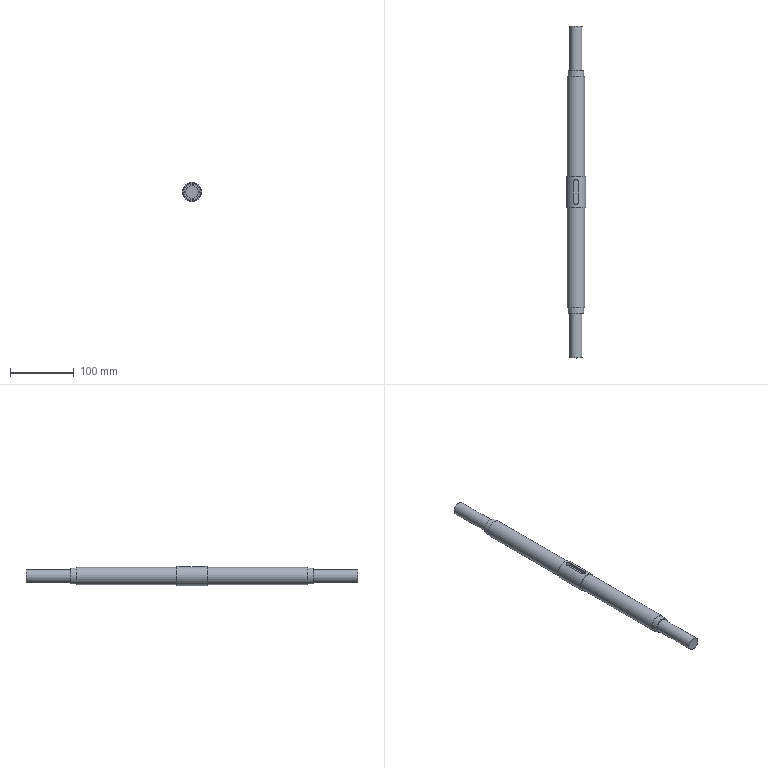Part | NX | features DATUM_CSYS 3, SKETCH 2, EXTRUDE 1, SWP104 1 | 1 solid | 20 faces | box 30 x 520 x 30 mm | volume 265320 mm3 | plane 11 | cylinder 9 | commonest cylinder face diameters 8 x2 20 x2 25 x2 27 x2 30 x1
STEP:
#1=CARTESIAN_POINT('',(0.,235.,15.));
#2=VERTEX_POINT('',#1);
#3=CARTESIAN_POINT('',(0.,235.,0.));
#4=DIRECTION('',(0.,1.,0.));
#5=DIRECTION('',(0.,0.,1.));
#6=AXIS2_PLACEMENT_3D('',#3,#4,#5);
#7=CIRCLE('',#6,15.);
#8=EDGE_CURVE('',#2,#2,#7,.T.);
#9=ORIENTED_EDGE('',*,*,#8,.T.);
#10=EDGE_LOOP('',(#9));
#11=FACE_BOUND('',#10,.T.);
#12=CARTESIAN_POINT('',(0.,285.,15.));
#13=VERTEX_POINT('',#12);
#14=CARTESIAN_POINT('',(0.,285.,0.));
#15=DIRECTION('',(0.,1.,0.));
#16=DIRECTION('',(0.,0.,1.));
#17=AXIS2_PLACEMENT_3D('',#14,#15,#16);
#18=CIRCLE('',#17,15.);
#19=EDGE_CURVE('',#13,#13,#18,.T.);
#20=ORIENTED_EDGE('',*,*,#19,.F.);
#21=EDGE_LOOP('',(#20));
#22=FACE_BOUND('',#21,.T.);
#23=CARTESIAN_POINT('',(-4.,276.,14.457));
#24=VERTEX_POINT('',#23);
#25=CARTESIAN_POINT('',(-4.,244.,14.457));
#26=VERTEX_POINT('',#25);
#27=CARTESIAN_POINT('',(-4.,0.,14.457));
#28=DIRECTION('',(0.,1.,0.));
#29=VECTOR('',#28,1000.);
#30=LINE('',#27,#29);
#31=EDGE_CURVE('',#24,#26,#30,.F.);
#32=ORIENTED_EDGE('',*,*,#31,.F.);
#33=CARTESIAN_POINT('',(4.,276.,14.457));
#34=VERTEX_POINT('',#33);
#35=CARTESIAN_POINT('',(4.,276.,14.457));
#36=CARTESIAN_POINT('',(4.,277.062,14.457));
#37=CARTESIAN_POINT('',(3.133,279.126,14.733));
#38=CARTESIAN_POINT('',(0.005849,280.437,15.133));
#39=CARTESIAN_POINT('',(-3.134,279.128,14.734));
#40=CARTESIAN_POINT('',(-4.,277.062,14.457));
#41=CARTESIAN_POINT('',(-4.,276.,14.457));
#42=B_SPLINE_CURVE_WITH_KNOTS('',3,(#35,#36,#37,#38,#39,#40,#41),.UNSPECIFIED.,.F.,.F.,(4,1,1,1,4),(0.,0.00314,0.006279,0.009419,0.01256),.UNSPECIFIED.);
#43=EDGE_CURVE('',#34,#24,#42,.T.);
#44=ORIENTED_EDGE('',*,*,#43,.F.);
#45=CARTESIAN_POINT('',(4.,244.,14.457));
#46=VERTEX_POINT('',#45);
#47=CARTESIAN_POINT('',(4.,0.,14.457));
#48=DIRECTION('',(0.,1.,0.));
#49=VECTOR('',#48,1000.);
#50=LINE('',#47,#49);
#51=EDGE_CURVE('',#46,#34,#50,.T.);
#52=ORIENTED_EDGE('',*,*,#51,.F.);
#53=CARTESIAN_POINT('',(-4.,244.,14.457));
#54=CARTESIAN_POINT('',(-4.,242.938,14.457));
#55=CARTESIAN_POINT('',(-3.133,240.874,14.733));
#56=CARTESIAN_POINT('',(-0.005849,239.563,15.133));
#57=CARTESIAN_POINT('',(3.134,240.872,14.734));
#58=CARTESIAN_POINT('',(4.,242.938,14.457));
#59=CARTESIAN_POINT('',(4.,244.,14.457));
#60=B_SPLINE_CURVE_WITH_KNOTS('',3,(#53,#54,#55,#56,#57,#58,#59),.UNSPECIFIED.,.F.,.F.,(4,1,1,1,4),(0.,0.00314,0.006279,0.009419,0.01256),.UNSPECIFIED.);
#61=EDGE_CURVE('',#26,#46,#60,.T.);
#62=ORIENTED_EDGE('',*,*,#61,.F.);
#63=EDGE_LOOP('',(#32,#44,#52,#62));
#64=FACE_BOUND('',#63,.T.);
#65=CARTESIAN_POINT('',(0.,0.,0.));
#66=DIRECTION('',(0.,1.,0.));
#67=DIRECTION('',(0.,0.,1.));
#68=AXIS2_PLACEMENT_3D('',#65,#66,#67);
#69=CYLINDRICAL_SURFACE('',#68,15.);
#70=ADVANCED_FACE('',(#11,#22,#64),#69,.T.);
#71=CARTESIAN_POINT('',(0.,0.,10.));
#72=VERTEX_POINT('',#71);
#73=CARTESIAN_POINT('',(0.,0.,0.));
#74=DIRECTION('',(0.,1.,0.));
#75=DIRECTION('',(0.,0.,1.));
#76=AXIS2_PLACEMENT_3D('',#73,#74,#75);
#77=CIRCLE('',#76,10.);
#78=EDGE_CURVE('',#72,#72,#77,.T.);
#79=ORIENTED_EDGE('',*,*,#78,.F.);
#80=EDGE_LOOP('',(#79));
#81=FACE_BOUND('',#80,.T.);
#82=CARTESIAN_POINT('',(0.,0.,0.));
#83=DIRECTION('',(0.,1.,0.));
#84=DIRECTION('',(0.,0.,1.));
#85=AXIS2_PLACEMENT_3D('',#82,#83,#84);
#86=PLANE('',#85);
#87=ADVANCED_FACE('',(#81),#86,.F.);
#88=CARTESIAN_POINT('',(0.,520.,10.));
#89=VERTEX_POINT('',#88);
#90=CARTESIAN_POINT('',(0.,520.,0.));
#91=DIRECTION('',(0.,1.,0.));
#92=DIRECTION('',(0.,0.,1.));
#93=AXIS2_PLACEMENT_3D('',#90,#91,#92);
#94=CIRCLE('',#93,10.);
#95=EDGE_CURVE('',#89,#89,#94,.T.);
#96=ORIENTED_EDGE('',*,*,#95,.T.);
#97=EDGE_LOOP('',(#96));
#98=FACE_BOUND('',#97,.T.);
#99=CARTESIAN_POINT('',(0.,520.,0.));
#100=DIRECTION('',(0.,1.,0.));
#101=DIRECTION('',(0.,0.,1.));
#102=AXIS2_PLACEMENT_3D('',#99,#100,#101);
#103=PLANE('',#102);
#104=ADVANCED_FACE('',(#98),#103,.T.);
#105=ORIENTED_EDGE('',*,*,#95,.F.);
#106=EDGE_LOOP('',(#105));
#107=FACE_BOUND('',#106,.T.);
#108=CARTESIAN_POINT('',(0.,450.,10.));
#109=VERTEX_POINT('',#108);
#110=CARTESIAN_POINT('',(0.,450.,0.));
#111=DIRECTION('',(0.,1.,0.));
#112=DIRECTION('',(0.,0.,1.));
#113=AXIS2_PLACEMENT_3D('',#110,#111,#112);
#114=CIRCLE('',#113,10.);
#115=EDGE_CURVE('',#109,#109,#114,.T.);
#116=ORIENTED_EDGE('',*,*,#115,.T.);
#117=EDGE_LOOP('',(#116));
#118=FACE_BOUND('',#117,.T.);
#119=CARTESIAN_POINT('',(0.,0.,0.));
#120=DIRECTION('',(0.,1.,0.));
#121=DIRECTION('',(0.,0.,1.));
#122=AXIS2_PLACEMENT_3D('',#119,#120,#121);
#123=CYLINDRICAL_SURFACE('',#122,10.);
#124=ADVANCED_FACE('',(#107,#118),#123,.T.);
#125=ORIENTED_EDGE('',*,*,#115,.F.);
#126=EDGE_LOOP('',(#125));
#127=FACE_BOUND('',#126,.T.);
#128=CARTESIAN_POINT('',(0.,450.,12.5));
#129=VERTEX_POINT('',#128);
#130=CARTESIAN_POINT('',(0.,450.,0.));
#131=DIRECTION('',(0.,1.,0.));
#132=DIRECTION('',(0.,0.,1.));
#133=AXIS2_PLACEMENT_3D('',#130,#131,#132);
#134=CIRCLE('',#133,12.5);
#135=EDGE_CURVE('',#129,#129,#134,.T.);
#136=ORIENTED_EDGE('',*,*,#135,.T.);
#137=EDGE_LOOP('',(#136));
#138=FACE_BOUND('',#137,.T.);
#139=CARTESIAN_POINT('',(-12.5,450.,0.));
#140=DIRECTION('',(0.,-1.,0.));
#141=DIRECTION('',(0.,0.,-1.));
#142=AXIS2_PLACEMENT_3D('',#139,#140,#141);
#143=PLANE('',#142);
#144=ADVANCED_FACE('',(#127,#138),#143,.F.);
#145=ORIENTED_EDGE('',*,*,#135,.F.);
#146=EDGE_LOOP('',(#145));
#147=FACE_BOUND('',#146,.T.);
#148=CARTESIAN_POINT('',(0.,441.,12.5));
#149=VERTEX_POINT('',#148);
#150=CARTESIAN_POINT('',(0.,441.,0.));
#151=DIRECTION('',(0.,1.,0.));
#152=DIRECTION('',(0.,0.,1.));
#153=AXIS2_PLACEMENT_3D('',#150,#151,#152);
#154=CIRCLE('',#153,12.5);
#155=EDGE_CURVE('',#149,#149,#154,.T.);
#156=ORIENTED_EDGE('',*,*,#155,.T.);
#157=EDGE_LOOP('',(#156));
#158=FACE_BOUND('',#157,.T.);
#159=CARTESIAN_POINT('',(0.,0.,0.));
#160=DIRECTION('',(0.,1.,0.));
#161=DIRECTION('',(0.,0.,1.));
#162=AXIS2_PLACEMENT_3D('',#159,#160,#161);
#163=CYLINDRICAL_SURFACE('',#162,12.5);
#164=ADVANCED_FACE('',(#147,#158),#163,.T.);
#165=ORIENTED_EDGE('',*,*,#155,.F.);
#166=EDGE_LOOP('',(#165));
#167=FACE_BOUND('',#166,.T.);
#168=CARTESIAN_POINT('',(0.,441.,13.5));
#169=VERTEX_POINT('',#168);
#170=CARTESIAN_POINT('',(0.,441.,0.));
#171=DIRECTION('',(0.,1.,0.));
#172=DIRECTION('',(0.,0.,1.));
#173=AXIS2_PLACEMENT_3D('',#170,#171,#172);
#174=CIRCLE('',#173,13.5);
#175=EDGE_CURVE('',#169,#169,#174,.T.);
#176=ORIENTED_EDGE('',*,*,#175,.T.);
#177=EDGE_LOOP('',(#176));
#178=FACE_BOUND('',#177,.T.);
#179=CARTESIAN_POINT('',(-13.5,441.,0.));
#180=DIRECTION('',(0.,-1.,0.));
#181=DIRECTION('',(0.,0.,-1.));
#182=AXIS2_PLACEMENT_3D('',#179,#180,#181);
#183=PLANE('',#182);
#184=ADVANCED_FACE('',(#167,#178),#183,.F.);
#185=ORIENTED_EDGE('',*,*,#175,.F.);
#186=EDGE_LOOP('',(#185));
#187=FACE_BOUND('',#186,.T.);
#188=CARTESIAN_POINT('',(0.,285.,13.5));
#189=VERTEX_POINT('',#188);
#190=CARTESIAN_POINT('',(0.,285.,0.));
#191=DIRECTION('',(0.,1.,0.));
#192=DIRECTION('',(0.,0.,1.));
#193=AXIS2_PLACEMENT_3D('',#190,#191,#192);
#194=CIRCLE('',#193,13.5);
#195=EDGE_CURVE('',#189,#189,#194,.T.);
#196=ORIENTED_EDGE('',*,*,#195,.T.);
#197=EDGE_LOOP('',(#196));
#198=FACE_BOUND('',#197,.T.);
#199=CARTESIAN_POINT('',(0.,0.,0.));
#200=DIRECTION('',(0.,1.,0.));
#201=DIRECTION('',(0.,0.,1.));
#202=AXIS2_PLACEMENT_3D('',#199,#200,#201);
#203=CYLINDRICAL_SURFACE('',#202,13.5);
#204=ADVANCED_FACE('',(#187,#198),#203,.T.);
#205=ORIENTED_EDGE('',*,*,#195,.F.);
#206=EDGE_LOOP('',(#205));
#207=FACE_BOUND('',#206,.T.);
#208=ORIENTED_EDGE('',*,*,#19,.T.);
#209=EDGE_LOOP('',(#208));
#210=FACE_BOUND('',#209,.T.);
#211=CARTESIAN_POINT('',(-15.,285.,0.));
#212=DIRECTION('',(0.,-1.,0.));
#213=DIRECTION('',(0.,0.,-1.));
#214=AXIS2_PLACEMENT_3D('',#211,#212,#213);
#215=PLANE('',#214);
#216=ADVANCED_FACE('',(#207,#210),#215,.F.);
#217=ORIENTED_EDGE('',*,*,#8,.F.);
#218=EDGE_LOOP('',(#217));
#219=FACE_BOUND('',#218,.T.);
#220=CARTESIAN_POINT('',(0.,235.,13.5));
#221=VERTEX_POINT('',#220);
#222=CARTESIAN_POINT('',(0.,235.,0.));
#223=DIRECTION('',(0.,1.,0.));
#224=DIRECTION('',(0.,0.,1.));
#225=AXIS2_PLACEMENT_3D('',#222,#223,#224);
#226=CIRCLE('',#225,13.5);
#227=EDGE_CURVE('',#221,#221,#226,.T.);
#228=ORIENTED_EDGE('',*,*,#227,.T.);
#229=EDGE_LOOP('',(#228));
#230=FACE_BOUND('',#229,.T.);
#231=CARTESIAN_POINT('',(-13.5,235.,0.));
#232=DIRECTION('',(0.,1.,0.));
#233=DIRECTION('',(0.,0.,1.));
#234=AXIS2_PLACEMENT_3D('',#231,#232,#233);
#235=PLANE('',#234);
#236=ADVANCED_FACE('',(#219,#230),#235,.F.);
#237=ORIENTED_EDGE('',*,*,#227,.F.);
#238=EDGE_LOOP('',(#237));
#239=FACE_BOUND('',#238,.T.);
#240=CARTESIAN_POINT('',(0.,79.,13.5));
#241=VERTEX_POINT('',#240);
#242=CARTESIAN_POINT('',(0.,79.,0.));
#243=DIRECTION('',(0.,1.,0.));
#244=DIRECTION('',(0.,0.,1.));
#245=AXIS2_PLACEMENT_3D('',#242,#243,#244);
#246=CIRCLE('',#245,13.5);
#247=EDGE_CURVE('',#241,#241,#246,.T.);
#248=ORIENTED_EDGE('',*,*,#247,.T.);
#249=EDGE_LOOP('',(#248));
#250=FACE_BOUND('',#249,.T.);
#251=CARTESIAN_POINT('',(0.,0.,0.));
#252=DIRECTION('',(0.,1.,0.));
#253=DIRECTION('',(0.,0.,1.));
#254=AXIS2_PLACEMENT_3D('',#251,#252,#253);
#255=CYLINDRICAL_SURFACE('',#254,13.5);
#256=ADVANCED_FACE('',(#239,#250),#255,.T.);
#257=ORIENTED_EDGE('',*,*,#247,.F.);
#258=EDGE_LOOP('',(#257));
#259=FACE_BOUND('',#258,.T.);
#260=CARTESIAN_POINT('',(0.,79.,12.5));
#261=VERTEX_POINT('',#260);
#262=CARTESIAN_POINT('',(0.,79.,0.));
#263=DIRECTION('',(0.,1.,0.));
#264=DIRECTION('',(0.,0.,1.));
#265=AXIS2_PLACEMENT_3D('',#262,#263,#264);
#266=CIRCLE('',#265,12.5);
#267=EDGE_CURVE('',#261,#261,#266,.T.);
#268=ORIENTED_EDGE('',*,*,#267,.T.);
#269=EDGE_LOOP('',(#268));
#270=FACE_BOUND('',#269,.T.);
#271=CARTESIAN_POINT('',(-12.5,79.,0.));
#272=DIRECTION('',(0.,1.,0.));
#273=DIRECTION('',(0.,0.,1.));
#274=AXIS2_PLACEMENT_3D('',#271,#272,#273);
#275=PLANE('',#274);
#276=ADVANCED_FACE('',(#259,#270),#275,.F.);
#277=ORIENTED_EDGE('',*,*,#267,.F.);
#278=EDGE_LOOP('',(#277));
#279=FACE_BOUND('',#278,.T.);
#280=CARTESIAN_POINT('',(0.,70.,12.5));
#281=VERTEX_POINT('',#280);
#282=CARTESIAN_POINT('',(0.,70.,0.));
#283=DIRECTION('',(0.,1.,0.));
#284=DIRECTION('',(0.,0.,1.));
#285=AXIS2_PLACEMENT_3D('',#282,#283,#284);
#286=CIRCLE('',#285,12.5);
#287=EDGE_CURVE('',#281,#281,#286,.T.);
#288=ORIENTED_EDGE('',*,*,#287,.T.);
#289=EDGE_LOOP('',(#288));
#290=FACE_BOUND('',#289,.T.);
#291=CARTESIAN_POINT('',(0.,0.,0.));
#292=DIRECTION('',(0.,1.,0.));
#293=DIRECTION('',(0.,0.,1.));
#294=AXIS2_PLACEMENT_3D('',#291,#292,#293);
#295=CYLINDRICAL_SURFACE('',#294,12.5);
#296=ADVANCED_FACE('',(#279,#290),#295,.T.);
#297=ORIENTED_EDGE('',*,*,#287,.F.);
#298=EDGE_LOOP('',(#297));
#299=FACE_BOUND('',#298,.T.);
#300=CARTESIAN_POINT('',(0.,70.,10.));
#301=VERTEX_POINT('',#300);
#302=CARTESIAN_POINT('',(0.,70.,0.));
#303=DIRECTION('',(0.,1.,0.));
#304=DIRECTION('',(0.,0.,1.));
#305=AXIS2_PLACEMENT_3D('',#302,#303,#304);
#306=CIRCLE('',#305,10.);
#307=EDGE_CURVE('',#301,#301,#306,.T.);
#308=ORIENTED_EDGE('',*,*,#307,.T.);
#309=EDGE_LOOP('',(#308));
#310=FACE_BOUND('',#309,.T.);
#311=CARTESIAN_POINT('',(-10.,70.,0.));
#312=DIRECTION('',(0.,1.,0.));
#313=DIRECTION('',(0.,0.,1.));
#314=AXIS2_PLACEMENT_3D('',#311,#312,#313);
#315=PLANE('',#314);
#316=ADVANCED_FACE('',(#299,#310),#315,.F.);
#317=ORIENTED_EDGE('',*,*,#307,.F.);
#318=EDGE_LOOP('',(#317));
#319=FACE_BOUND('',#318,.T.);
#320=ORIENTED_EDGE('',*,*,#78,.T.);
#321=EDGE_LOOP('',(#320));
#322=FACE_BOUND('',#321,.T.);
#323=CARTESIAN_POINT('',(0.,0.,0.));
#324=DIRECTION('',(0.,1.,0.));
#325=DIRECTION('',(0.,0.,1.));
#326=AXIS2_PLACEMENT_3D('',#323,#324,#325);
#327=CYLINDRICAL_SURFACE('',#326,10.);
#328=ADVANCED_FACE('',(#319,#322),#327,.T.);
#329=ORIENTED_EDGE('',*,*,#31,.T.);
#330=CARTESIAN_POINT('',(-4.,244.,10.));
#331=VERTEX_POINT('',#330);
#332=CARTESIAN_POINT('',(-4.,244.,32.));
#333=DIRECTION('',(0.,0.,-1.));
#334=VECTOR('',#333,1000.);
#335=LINE('',#332,#334);
#336=EDGE_CURVE('',#331,#26,#335,.F.);
#337=ORIENTED_EDGE('',*,*,#336,.F.);
#338=CARTESIAN_POINT('',(-4.,276.,10.));
#339=VERTEX_POINT('',#338);
#340=CARTESIAN_POINT('',(-4.,276.,10.));
#341=DIRECTION('',(0.,-1.,0.));
#342=VECTOR('',#341,1000.);
#343=LINE('',#340,#342);
#344=EDGE_CURVE('',#331,#339,#343,.F.);
#345=ORIENTED_EDGE('',*,*,#344,.T.);
#346=CARTESIAN_POINT('',(-4.,276.,32.));
#347=DIRECTION('',(0.,0.,-1.));
#348=VECTOR('',#347,1000.);
#349=LINE('',#346,#348);
#350=EDGE_CURVE('',#339,#24,#349,.F.);
#351=ORIENTED_EDGE('',*,*,#350,.T.);
#352=EDGE_LOOP('',(#329,#337,#345,#351));
#353=FACE_BOUND('',#352,.T.);
#354=CARTESIAN_POINT('',(-4.,276.,32.));
#355=DIRECTION('',(1.,0.,0.));
#356=DIRECTION('',(0.,1.,0.));
#357=AXIS2_PLACEMENT_3D('',#354,#355,#356);
#358=PLANE('',#357);
#359=ADVANCED_FACE('',(#353),#358,.T.);
#360=ORIENTED_EDGE('',*,*,#61,.T.);
#361=CARTESIAN_POINT('',(4.,244.,10.));
#362=VERTEX_POINT('',#361);
#363=CARTESIAN_POINT('',(4.,244.,32.));
#364=DIRECTION('',(0.,0.,-1.));
#365=VECTOR('',#364,1000.);
#366=LINE('',#363,#365);
#367=EDGE_CURVE('',#362,#46,#366,.F.);
#368=ORIENTED_EDGE('',*,*,#367,.F.);
#369=CARTESIAN_POINT('',(0.,244.,10.));
#370=DIRECTION('',(0.,0.,1.));
#371=DIRECTION('',(1.,0.,0.));
#372=AXIS2_PLACEMENT_3D('',#369,#370,#371);
#373=CIRCLE('',#372,4.);
#374=EDGE_CURVE('',#362,#331,#373,.F.);
#375=ORIENTED_EDGE('',*,*,#374,.T.);
#376=ORIENTED_EDGE('',*,*,#336,.T.);
#377=EDGE_LOOP('',(#360,#368,#375,#376));
#378=FACE_BOUND('',#377,.T.);
#379=CARTESIAN_POINT('',(0.,244.,32.));
#380=DIRECTION('',(0.,0.,-1.));
#381=DIRECTION('',(-1.,0.,0.));
#382=AXIS2_PLACEMENT_3D('',#379,#380,#381);
#383=CYLINDRICAL_SURFACE('',#382,4.);
#384=ADVANCED_FACE('',(#378),#383,.F.);
#385=ORIENTED_EDGE('',*,*,#51,.T.);
#386=CARTESIAN_POINT('',(4.,276.,10.));
#387=VERTEX_POINT('',#386);
#388=CARTESIAN_POINT('',(4.,276.,32.));
#389=DIRECTION('',(0.,0.,-1.));
#390=VECTOR('',#389,1000.);
#391=LINE('',#388,#390);
#392=EDGE_CURVE('',#387,#34,#391,.F.);
#393=ORIENTED_EDGE('',*,*,#392,.F.);
#394=CARTESIAN_POINT('',(4.,244.,10.));
#395=DIRECTION('',(0.,1.,0.));
#396=VECTOR('',#395,1000.);
#397=LINE('',#394,#396);
#398=EDGE_CURVE('',#387,#362,#397,.F.);
#399=ORIENTED_EDGE('',*,*,#398,.T.);
#400=ORIENTED_EDGE('',*,*,#367,.T.);
#401=EDGE_LOOP('',(#385,#393,#399,#400));
#402=FACE_BOUND('',#401,.T.);
#403=CARTESIAN_POINT('',(4.,244.,32.));
#404=DIRECTION('',(-1.,0.,0.));
#405=DIRECTION('',(0.,0.,1.));
#406=AXIS2_PLACEMENT_3D('',#403,#404,#405);
#407=PLANE('',#406);
#408=ADVANCED_FACE('',(#402),#407,.T.);
#409=ORIENTED_EDGE('',*,*,#43,.T.);
#410=ORIENTED_EDGE('',*,*,#350,.F.);
#411=CARTESIAN_POINT('',(0.,276.,10.));
#412=DIRECTION('',(0.,0.,1.));
#413=DIRECTION('',(1.,0.,0.));
#414=AXIS2_PLACEMENT_3D('',#411,#412,#413);
#415=CIRCLE('',#414,4.);
#416=EDGE_CURVE('',#339,#387,#415,.F.);
#417=ORIENTED_EDGE('',*,*,#416,.T.);
#418=ORIENTED_EDGE('',*,*,#392,.T.);
#419=EDGE_LOOP('',(#409,#410,#417,#418));
#420=FACE_BOUND('',#419,.T.);
#421=CARTESIAN_POINT('',(0.,276.,32.));
#422=DIRECTION('',(0.,0.,-1.));
#423=DIRECTION('',(-1.,0.,0.));
#424=AXIS2_PLACEMENT_3D('',#421,#422,#423);
#425=CYLINDRICAL_SURFACE('',#424,4.);
#426=ADVANCED_FACE('',(#420),#425,.F.);
#427=ORIENTED_EDGE('',*,*,#344,.F.);
#428=ORIENTED_EDGE('',*,*,#374,.F.);
#429=ORIENTED_EDGE('',*,*,#398,.F.);
#430=ORIENTED_EDGE('',*,*,#416,.F.);
#431=EDGE_LOOP('',(#427,#428,#429,#430));
#432=FACE_BOUND('',#431,.T.);
#433=CARTESIAN_POINT('',(0.,244.,10.));
#434=DIRECTION('',(0.,0.,1.));
#435=DIRECTION('',(1.,0.,0.));
#436=AXIS2_PLACEMENT_3D('',#433,#434,#435);
#437=PLANE('',#436);
#438=ADVANCED_FACE('',(#432),#437,.T.);
#439=CLOSED_SHELL('',(#70,#87,#104,#124,#144,#164,#184,#204,#216,#236,#256,#276,#296,#316,#328,#359,#384,#408,#426,#438));
#440=MANIFOLD_SOLID_BREP('',#439);
#441=(LENGTH_UNIT()NAMED_UNIT(*)SI_UNIT(.MILLI.,.METRE.));
#442=UNCERTAINTY_MEASURE_WITH_UNIT(LENGTH_MEASURE(0.0508),#441,'','');
#443=(NAMED_UNIT(*)PLANE_ANGLE_UNIT()SI_UNIT($,.RADIAN.));
#444=(NAMED_UNIT(*)SI_UNIT($,.STERADIAN.)SOLID_ANGLE_UNIT());
#445=(GEOMETRIC_REPRESENTATION_CONTEXT(3)GLOBAL_UNCERTAINTY_ASSIGNED_CONTEXT((#442))GLOBAL_UNIT_ASSIGNED_CONTEXT((#441,#443,#444))REPRESENTATION_CONTEXT('',''));
#446=ADVANCED_BREP_SHAPE_REPRESENTATION('',(#440),#445);